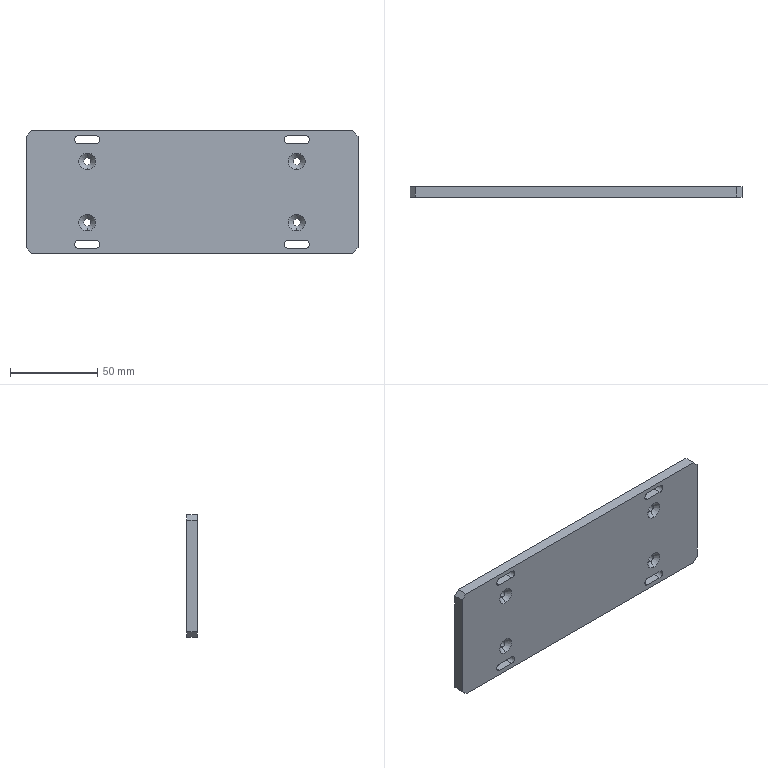Part | STEP file | PN_0027 | 1 solid | 42 faces | box 190 x 6 x 70 mm | volume 77614 mm3 | plane 18 | cylinder 16 | cone 8 | commonest cylinder face diameters 4.3 x8 4.5 x8